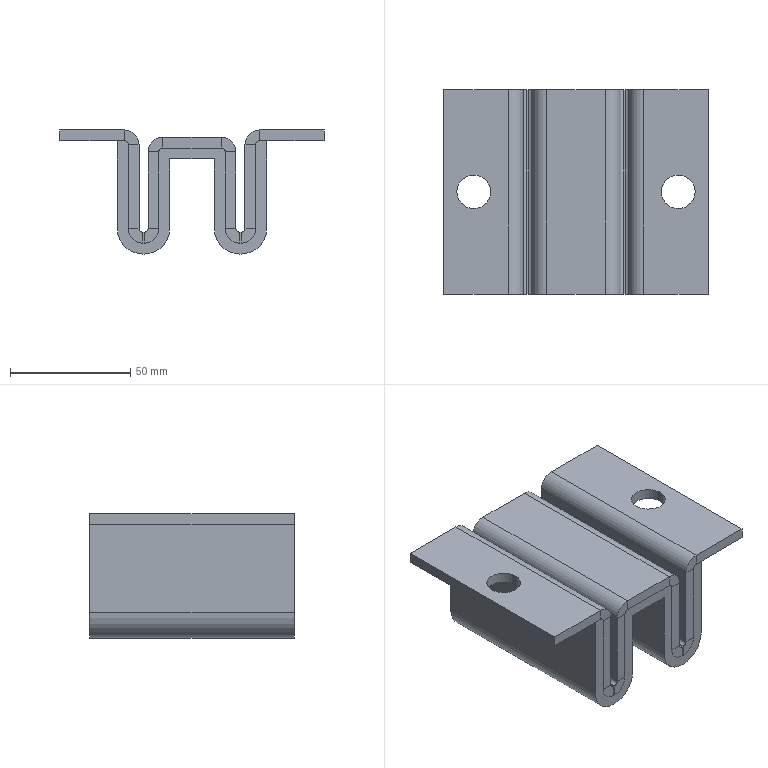Part | STEP file | TK5 guide rail single shoe head | 2 solids | 104 faces | box 110 x 85 x 51.5 mm | volume 179270 mm3 | plane 72 | cylinder 32 | commonest cylinder face diameters 3.08 x12 12.08 x12 14 x4 21.08 x4